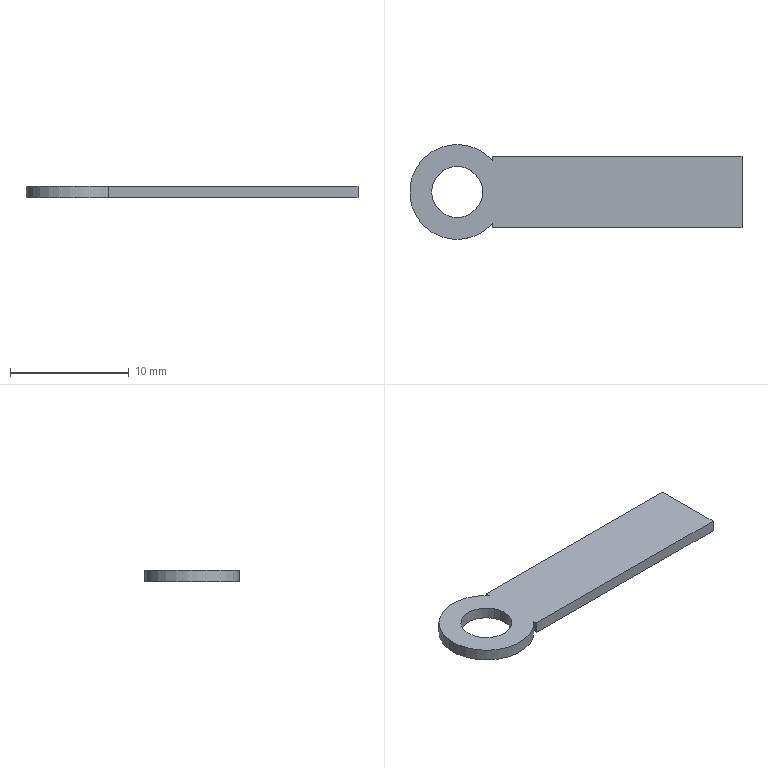Part | SolidWorks | features Extrusion 1, ICE 1 | 1 solid | 10 faces | box 28 x 8 x 1 mm | volume 158.117 mm3 | plane 7 | cylinder 3 | commonest cylinder face diameters 4.3 x2 8 x1
STEP:
#1=CARTESIAN_POINT('',(-2.15,0.,-0.5));
#2=VERTEX_POINT('',#1);
#3=CARTESIAN_POINT('',(2.15,0.,-0.5));
#4=VERTEX_POINT('',#3);
#5=CARTESIAN_POINT('',(0.,0.,-0.5));
#6=DIRECTION('',(0.,0.,1.));
#7=DIRECTION('',(1.,0.,0.));
#8=AXIS2_PLACEMENT_3D('',#5,#6,#7);
#9=CIRCLE('',#8,2.15);
#10=EDGE_CURVE('',#2,#4,#9,.T.);
#11=ORIENTED_EDGE('',*,*,#10,.F.);
#12=CARTESIAN_POINT('',(-2.15,0.,0.5));
#13=VERTEX_POINT('',#12);
#14=CARTESIAN_POINT('',(-2.15,0.,-0.5));
#15=DIRECTION('',(0.,0.,1.));
#16=VECTOR('',#15,1000.);
#17=LINE('',#14,#16);
#18=EDGE_CURVE('',#2,#13,#17,.T.);
#19=ORIENTED_EDGE('',*,*,#18,.T.);
#20=CARTESIAN_POINT('',(2.15,0.,0.5));
#21=VERTEX_POINT('',#20);
#22=CARTESIAN_POINT('',(0.,0.,0.5));
#23=DIRECTION('',(0.,0.,1.));
#24=DIRECTION('',(1.,0.,0.));
#25=AXIS2_PLACEMENT_3D('',#22,#23,#24);
#26=CIRCLE('',#25,2.15);
#27=EDGE_CURVE('',#13,#21,#26,.T.);
#28=ORIENTED_EDGE('',*,*,#27,.T.);
#29=CARTESIAN_POINT('',(2.15,0.,-0.5));
#30=DIRECTION('',(0.,0.,1.));
#31=VECTOR('',#30,1000.);
#32=LINE('',#29,#31);
#33=EDGE_CURVE('',#4,#21,#32,.T.);
#34=ORIENTED_EDGE('',*,*,#33,.F.);
#35=EDGE_LOOP('',(#11,#19,#28,#34));
#36=FACE_OUTER_BOUND('',#35,.T.);
#37=CARTESIAN_POINT('',(0.,0.,-0.5));
#38=DIRECTION('',(0.,0.,1.));
#39=DIRECTION('',(1.,0.,0.));
#40=AXIS2_PLACEMENT_3D('',#37,#38,#39);
#41=CYLINDRICAL_SURFACE('',#40,2.15);
#42=ADVANCED_FACE('',(#36),#41,.F.);
#43=CARTESIAN_POINT('',(3.,-2.646,0.5));
#44=VERTEX_POINT('',#43);
#45=CARTESIAN_POINT('',(3.,-2.646,-0.5));
#46=VERTEX_POINT('',#45);
#47=CARTESIAN_POINT('',(3.,-2.646,-0.5));
#48=DIRECTION('',(0.,0.,-1.));
#49=VECTOR('',#48,1000.);
#50=LINE('',#47,#49);
#51=EDGE_CURVE('',#44,#46,#50,.T.);
#52=ORIENTED_EDGE('',*,*,#51,.F.);
#53=CARTESIAN_POINT('',(3.,2.646,0.5));
#54=VERTEX_POINT('',#53);
#55=CARTESIAN_POINT('',(0.,0.,0.5));
#56=DIRECTION('',(0.,0.,1.));
#57=DIRECTION('',(1.,0.,0.));
#58=AXIS2_PLACEMENT_3D('',#55,#56,#57);
#59=CIRCLE('',#58,4.);
#60=EDGE_CURVE('',#54,#44,#59,.T.);
#61=ORIENTED_EDGE('',*,*,#60,.F.);
#62=CARTESIAN_POINT('',(3.,2.646,-0.5));
#63=VERTEX_POINT('',#62);
#64=CARTESIAN_POINT('',(3.,2.646,-0.5));
#65=DIRECTION('',(0.,0.,1.));
#66=VECTOR('',#65,1000.);
#67=LINE('',#64,#66);
#68=EDGE_CURVE('',#63,#54,#67,.T.);
#69=ORIENTED_EDGE('',*,*,#68,.F.);
#70=CARTESIAN_POINT('',(0.,0.,-0.5));
#71=DIRECTION('',(0.,0.,1.));
#72=DIRECTION('',(1.,0.,0.));
#73=AXIS2_PLACEMENT_3D('',#70,#71,#72);
#74=CIRCLE('',#73,4.);
#75=EDGE_CURVE('',#63,#46,#74,.T.);
#76=ORIENTED_EDGE('',*,*,#75,.T.);
#77=EDGE_LOOP('',(#52,#61,#69,#76));
#78=FACE_OUTER_BOUND('',#77,.T.);
#79=CARTESIAN_POINT('',(0.,0.,-0.5));
#80=DIRECTION('',(0.,0.,1.));
#81=DIRECTION('',(1.,0.,0.));
#82=AXIS2_PLACEMENT_3D('',#79,#80,#81);
#83=CYLINDRICAL_SURFACE('',#82,4.);
#84=ADVANCED_FACE('',(#78),#83,.T.);
#85=CARTESIAN_POINT('',(0.,0.,-0.5));
#86=DIRECTION('',(0.,0.,1.));
#87=DIRECTION('',(1.,0.,0.));
#88=AXIS2_PLACEMENT_3D('',#85,#86,#87);
#89=CIRCLE('',#88,2.15);
#90=EDGE_CURVE('',#4,#2,#89,.T.);
#91=ORIENTED_EDGE('',*,*,#90,.T.);
#92=ORIENTED_EDGE('',*,*,#10,.T.);
#93=EDGE_LOOP('',(#91,#92));
#94=FACE_BOUND('',#93,.T.);
#95=ORIENTED_EDGE('',*,*,#75,.F.);
#96=CARTESIAN_POINT('',(3.,3.,-0.5));
#97=VERTEX_POINT('',#96);
#98=CARTESIAN_POINT('',(3.,3.,-0.5));
#99=DIRECTION('',(0.,-1.,0.));
#100=VECTOR('',#99,1000.);
#101=LINE('',#98,#100);
#102=EDGE_CURVE('',#97,#63,#101,.T.);
#103=ORIENTED_EDGE('',*,*,#102,.F.);
#104=CARTESIAN_POINT('',(24.,3.,-0.5));
#105=VERTEX_POINT('',#104);
#106=CARTESIAN_POINT('',(24.,3.,-0.5));
#107=DIRECTION('',(-1.,0.,0.));
#108=VECTOR('',#107,1000.);
#109=LINE('',#106,#108);
#110=EDGE_CURVE('',#105,#97,#109,.T.);
#111=ORIENTED_EDGE('',*,*,#110,.F.);
#112=CARTESIAN_POINT('',(24.,-3.,-0.5));
#113=VERTEX_POINT('',#112);
#114=CARTESIAN_POINT('',(24.,-3.,-0.5));
#115=DIRECTION('',(0.,1.,0.));
#116=VECTOR('',#115,1000.);
#117=LINE('',#114,#116);
#118=EDGE_CURVE('',#113,#105,#117,.T.);
#119=ORIENTED_EDGE('',*,*,#118,.F.);
#120=CARTESIAN_POINT('',(3.,-3.,-0.5));
#121=VERTEX_POINT('',#120);
#122=CARTESIAN_POINT('',(3.,-3.,-0.5));
#123=DIRECTION('',(1.,0.,0.));
#124=VECTOR('',#123,1000.);
#125=LINE('',#122,#124);
#126=EDGE_CURVE('',#121,#113,#125,.T.);
#127=ORIENTED_EDGE('',*,*,#126,.F.);
#128=CARTESIAN_POINT('',(3.,3.,-0.5));
#129=DIRECTION('',(0.,-1.,0.));
#130=VECTOR('',#129,1000.);
#131=LINE('',#128,#130);
#132=EDGE_CURVE('',#46,#121,#131,.T.);
#133=ORIENTED_EDGE('',*,*,#132,.F.);
#134=EDGE_LOOP('',(#95,#103,#111,#119,#127,#133));
#135=FACE_OUTER_BOUND('',#134,.T.);
#136=CARTESIAN_POINT('',(0.,0.,-0.5));
#137=DIRECTION('',(0.,0.,1.));
#138=DIRECTION('',(1.,0.,0.));
#139=AXIS2_PLACEMENT_3D('',#136,#137,#138);
#140=PLANE('',#139);
#141=ADVANCED_FACE('',(#94,#135),#140,.F.);
#142=ORIENTED_EDGE('',*,*,#60,.T.);
#143=CARTESIAN_POINT('',(3.,-3.,0.5));
#144=VERTEX_POINT('',#143);
#145=CARTESIAN_POINT('',(3.,3.,0.5));
#146=DIRECTION('',(0.,-1.,0.));
#147=VECTOR('',#146,1000.);
#148=LINE('',#145,#147);
#149=EDGE_CURVE('',#44,#144,#148,.T.);
#150=ORIENTED_EDGE('',*,*,#149,.T.);
#151=CARTESIAN_POINT('',(24.,-3.,0.5));
#152=VERTEX_POINT('',#151);
#153=CARTESIAN_POINT('',(3.,-3.,0.5));
#154=DIRECTION('',(1.,0.,0.));
#155=VECTOR('',#154,1000.);
#156=LINE('',#153,#155);
#157=EDGE_CURVE('',#144,#152,#156,.T.);
#158=ORIENTED_EDGE('',*,*,#157,.T.);
#159=CARTESIAN_POINT('',(24.,3.,0.5));
#160=VERTEX_POINT('',#159);
#161=CARTESIAN_POINT('',(24.,-3.,0.5));
#162=DIRECTION('',(0.,1.,0.));
#163=VECTOR('',#162,1000.);
#164=LINE('',#161,#163);
#165=EDGE_CURVE('',#152,#160,#164,.T.);
#166=ORIENTED_EDGE('',*,*,#165,.T.);
#167=CARTESIAN_POINT('',(3.,3.,0.5));
#168=VERTEX_POINT('',#167);
#169=CARTESIAN_POINT('',(24.,3.,0.5));
#170=DIRECTION('',(-1.,0.,0.));
#171=VECTOR('',#170,1000.);
#172=LINE('',#169,#171);
#173=EDGE_CURVE('',#160,#168,#172,.T.);
#174=ORIENTED_EDGE('',*,*,#173,.T.);
#175=CARTESIAN_POINT('',(3.,3.,0.5));
#176=DIRECTION('',(0.,-1.,0.));
#177=VECTOR('',#176,1000.);
#178=LINE('',#175,#177);
#179=EDGE_CURVE('',#168,#54,#178,.T.);
#180=ORIENTED_EDGE('',*,*,#179,.T.);
#181=EDGE_LOOP('',(#142,#150,#158,#166,#174,#180));
#182=FACE_OUTER_BOUND('',#181,.T.);
#183=CARTESIAN_POINT('',(0.,0.,0.5));
#184=DIRECTION('',(0.,0.,1.));
#185=DIRECTION('',(1.,0.,0.));
#186=AXIS2_PLACEMENT_3D('',#183,#184,#185);
#187=CIRCLE('',#186,2.15);
#188=EDGE_CURVE('',#21,#13,#187,.T.);
#189=ORIENTED_EDGE('',*,*,#188,.F.);
#190=ORIENTED_EDGE('',*,*,#27,.F.);
#191=EDGE_LOOP('',(#189,#190));
#192=FACE_BOUND('',#191,.T.);
#193=CARTESIAN_POINT('',(0.,0.,0.5));
#194=DIRECTION('',(0.,0.,1.));
#195=DIRECTION('',(1.,0.,0.));
#196=AXIS2_PLACEMENT_3D('',#193,#194,#195);
#197=PLANE('',#196);
#198=ADVANCED_FACE('',(#182,#192),#197,.T.);
#199=ORIENTED_EDGE('',*,*,#18,.F.);
#200=ORIENTED_EDGE('',*,*,#90,.F.);
#201=ORIENTED_EDGE('',*,*,#33,.T.);
#202=ORIENTED_EDGE('',*,*,#188,.T.);
#203=EDGE_LOOP('',(#199,#200,#201,#202));
#204=FACE_OUTER_BOUND('',#203,.T.);
#205=CARTESIAN_POINT('',(0.,0.,-0.5));
#206=DIRECTION('',(0.,0.,1.));
#207=DIRECTION('',(1.,0.,0.));
#208=AXIS2_PLACEMENT_3D('',#205,#206,#207);
#209=CYLINDRICAL_SURFACE('',#208,2.15);
#210=ADVANCED_FACE('',(#204),#209,.F.);
#211=ORIENTED_EDGE('',*,*,#149,.F.);
#212=ORIENTED_EDGE('',*,*,#51,.T.);
#213=ORIENTED_EDGE('',*,*,#132,.T.);
#214=CARTESIAN_POINT('',(3.,-3.,-0.5));
#215=DIRECTION('',(0.,0.,1.));
#216=VECTOR('',#215,1000.);
#217=LINE('',#214,#216);
#218=EDGE_CURVE('',#121,#144,#217,.T.);
#219=ORIENTED_EDGE('',*,*,#218,.T.);
#220=EDGE_LOOP('',(#211,#212,#213,#219));
#221=FACE_OUTER_BOUND('',#220,.T.);
#222=CARTESIAN_POINT('',(3.,3.,-0.5));
#223=DIRECTION('',(-1.,0.,0.));
#224=DIRECTION('',(0.,0.,1.));
#225=AXIS2_PLACEMENT_3D('',#222,#223,#224);
#226=PLANE('',#225);
#227=ADVANCED_FACE('',(#221),#226,.T.);
#228=ORIENTED_EDGE('',*,*,#102,.T.);
#229=ORIENTED_EDGE('',*,*,#68,.T.);
#230=ORIENTED_EDGE('',*,*,#179,.F.);
#231=CARTESIAN_POINT('',(3.,3.,-0.5));
#232=DIRECTION('',(0.,0.,1.));
#233=VECTOR('',#232,1000.);
#234=LINE('',#231,#233);
#235=EDGE_CURVE('',#97,#168,#234,.T.);
#236=ORIENTED_EDGE('',*,*,#235,.F.);
#237=EDGE_LOOP('',(#228,#229,#230,#236));
#238=FACE_OUTER_BOUND('',#237,.T.);
#239=CARTESIAN_POINT('',(3.,3.,-0.5));
#240=DIRECTION('',(-1.,0.,0.));
#241=DIRECTION('',(0.,0.,1.));
#242=AXIS2_PLACEMENT_3D('',#239,#240,#241);
#243=PLANE('',#242);
#244=ADVANCED_FACE('',(#238),#243,.T.);
#245=ORIENTED_EDGE('',*,*,#173,.F.);
#246=CARTESIAN_POINT('',(24.,3.,-0.5));
#247=DIRECTION('',(0.,0.,1.));
#248=VECTOR('',#247,1000.);
#249=LINE('',#246,#248);
#250=EDGE_CURVE('',#105,#160,#249,.T.);
#251=ORIENTED_EDGE('',*,*,#250,.F.);
#252=ORIENTED_EDGE('',*,*,#110,.T.);
#253=ORIENTED_EDGE('',*,*,#235,.T.);
#254=EDGE_LOOP('',(#245,#251,#252,#253));
#255=FACE_OUTER_BOUND('',#254,.T.);
#256=CARTESIAN_POINT('',(24.,3.,-0.5));
#257=DIRECTION('',(0.,1.,0.));
#258=DIRECTION('',(0.,0.,1.));
#259=AXIS2_PLACEMENT_3D('',#256,#257,#258);
#260=PLANE('',#259);
#261=ADVANCED_FACE('',(#255),#260,.T.);
#262=ORIENTED_EDGE('',*,*,#165,.F.);
#263=CARTESIAN_POINT('',(24.,-3.,-0.5));
#264=DIRECTION('',(0.,0.,1.));
#265=VECTOR('',#264,1000.);
#266=LINE('',#263,#265);
#267=EDGE_CURVE('',#113,#152,#266,.T.);
#268=ORIENTED_EDGE('',*,*,#267,.F.);
#269=ORIENTED_EDGE('',*,*,#118,.T.);
#270=ORIENTED_EDGE('',*,*,#250,.T.);
#271=EDGE_LOOP('',(#262,#268,#269,#270));
#272=FACE_OUTER_BOUND('',#271,.T.);
#273=CARTESIAN_POINT('',(24.,-3.,-0.5));
#274=DIRECTION('',(1.,0.,0.));
#275=DIRECTION('',(0.,0.,-1.));
#276=AXIS2_PLACEMENT_3D('',#273,#274,#275);
#277=PLANE('',#276);
#278=ADVANCED_FACE('',(#272),#277,.T.);
#279=ORIENTED_EDGE('',*,*,#157,.F.);
#280=ORIENTED_EDGE('',*,*,#218,.F.);
#281=ORIENTED_EDGE('',*,*,#126,.T.);
#282=ORIENTED_EDGE('',*,*,#267,.T.);
#283=EDGE_LOOP('',(#279,#280,#281,#282));
#284=FACE_OUTER_BOUND('',#283,.T.);
#285=CARTESIAN_POINT('',(3.,-3.,-0.5));
#286=DIRECTION('',(0.,-1.,0.));
#287=DIRECTION('',(0.,0.,-1.));
#288=AXIS2_PLACEMENT_3D('',#285,#286,#287);
#289=PLANE('',#288);
#290=ADVANCED_FACE('',(#284),#289,.T.);
#291=CLOSED_SHELL('',(#42,#84,#141,#198,#210,#227,#244,#261,#278,#290));
#292=MANIFOLD_SOLID_BREP('',#291);
#293=CARTESIAN_POINT('',(0.,0.,0.));
#294=DIRECTION('',(0.,0.,1.));
#295=DIRECTION('',(1.,0.,0.));
#296=AXIS2_PLACEMENT_3D('',#293,#294,#295);
#297=(LENGTH_UNIT()NAMED_UNIT(*)SI_UNIT(.MILLI.,.METRE.));
#298=UNCERTAINTY_MEASURE_WITH_UNIT(LENGTH_MEASURE(0.00001),#297,'','');
#299=(NAMED_UNIT(*)PLANE_ANGLE_UNIT()SI_UNIT($,.RADIAN.));
#300=(NAMED_UNIT(*)SI_UNIT($,.STERADIAN.)SOLID_ANGLE_UNIT());
#301=(GEOMETRIC_REPRESENTATION_CONTEXT(3)GLOBAL_UNCERTAINTY_ASSIGNED_CONTEXT((#298))GLOBAL_UNIT_ASSIGNED_CONTEXT((#297,#299,#300))REPRESENTATION_CONTEXT('',''));
#302=ADVANCED_BREP_SHAPE_REPRESENTATION('',(#292,#296),#301);